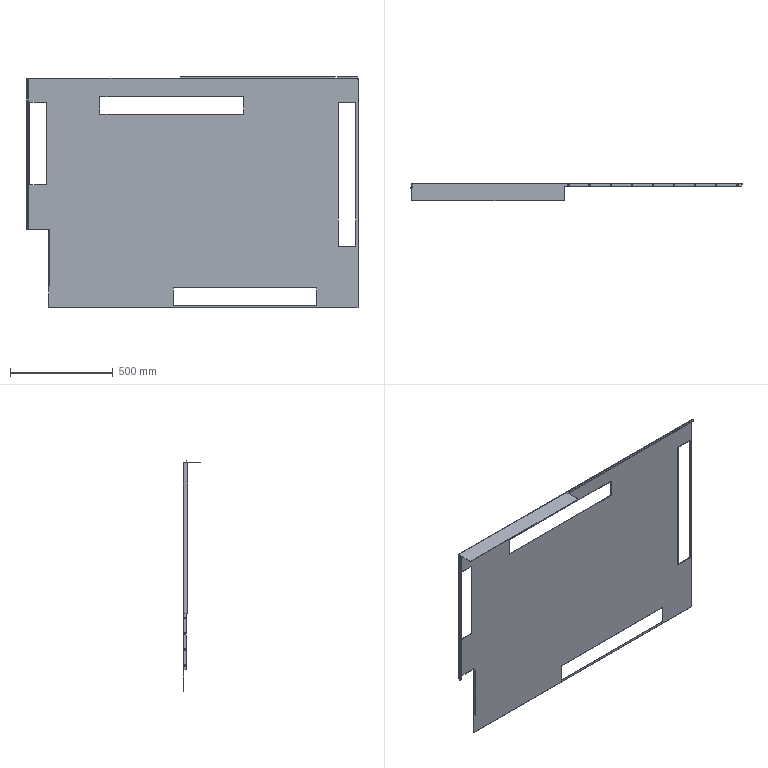Part | STEP file | Top Cover 1 | 1 solid | 96 faces | box 1618 x 85 x 1128 mm | volume 3307611 mm3 | plane 57 | cylinder 39 | commonest cylinder face diameters 6 x18 1 x8 7 x8 5 x5